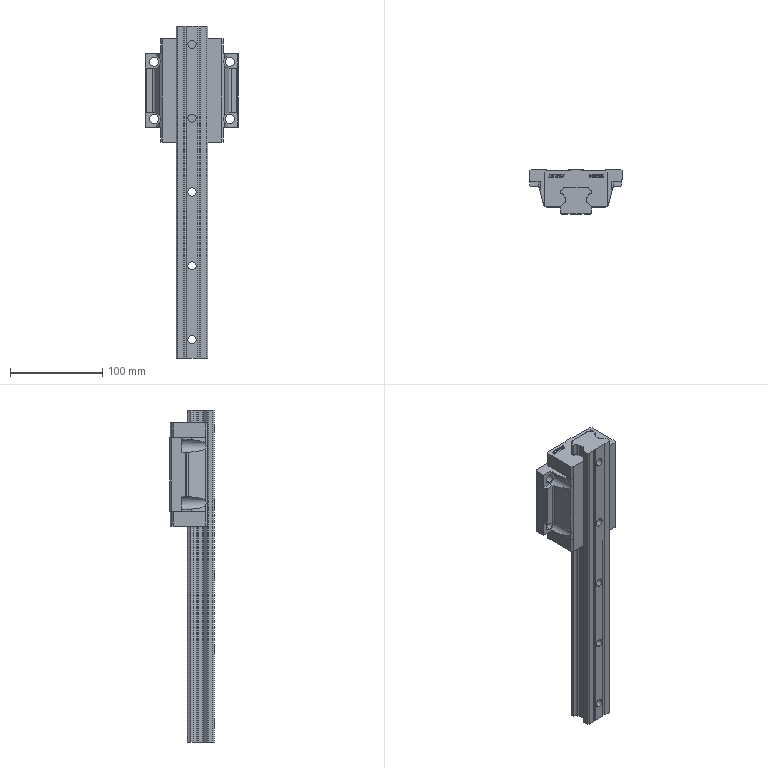Part | SolidWorks | 2 solids | 462 faces | box 100 x 48 x 360 mm | volume 575184 mm3 | plane 350 | spline 60 | cylinder 52 | commonest cylinder face diameters 2.4 x10 9 x10 14 x10 6.5 x8 10 x8 15 x4